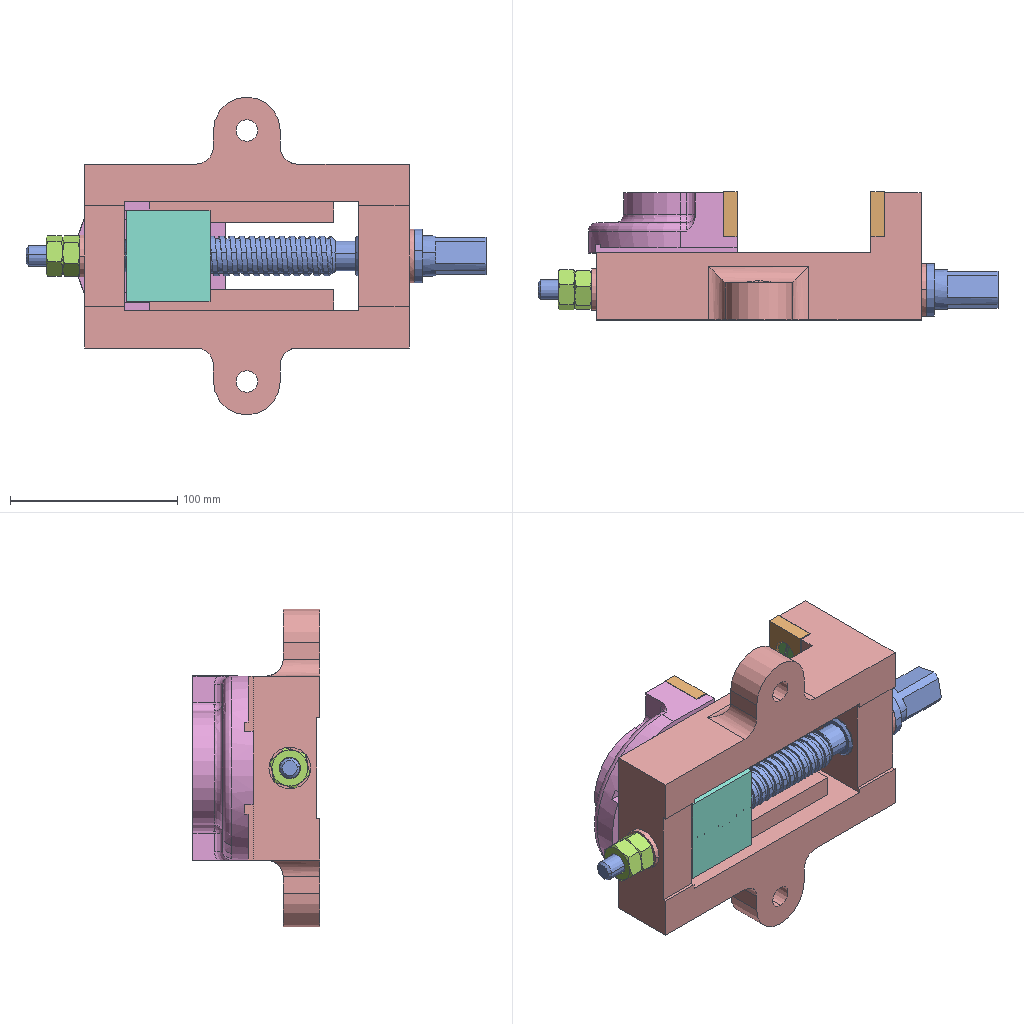Assembly | SolidWorks | 13 different items | 18 placed | box 275 x 76 x 190 mm
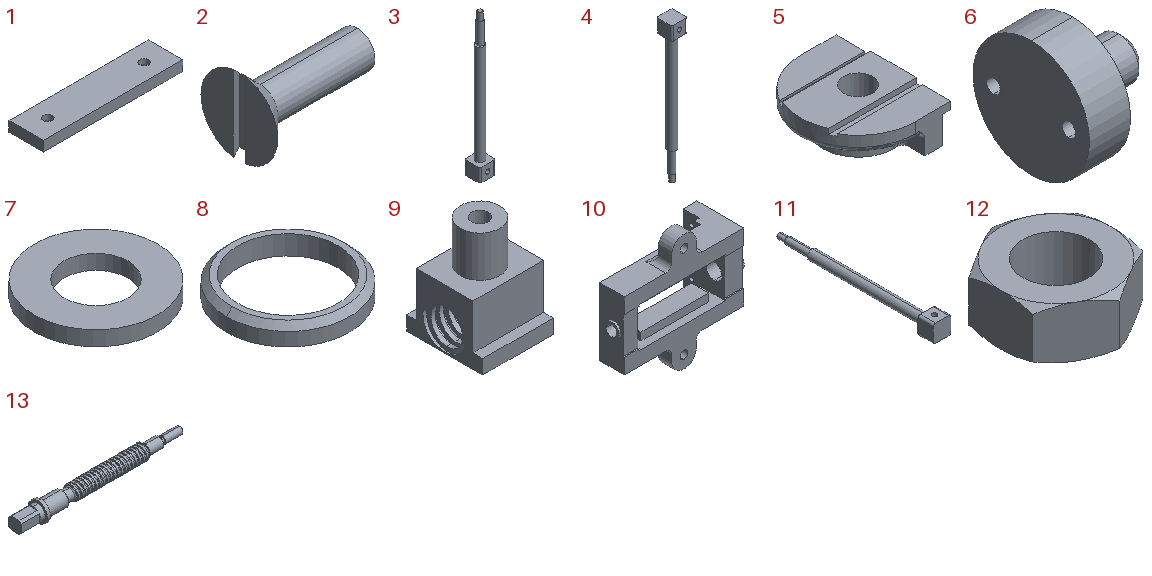Parts list (item | quantity | size | volume | features):
1 | x2 | 110 x 27 x 8 mm | 22658 mm3 | features Extrusion 1, MirrorPattern 1, RevCut 1
2 | x4 | 21.732 x 13 x 12.845 mm | 718.275 mm3 | features ICE 1, Revolution 1
3 | x1 | 40 x 40 x 370 mm | 162246 mm3 | features ICE 4, Chamfer 1, Extrusion 1
4 | x1 | 40 x 40 x 370 mm | 162450 mm3 | features ICE 4, Chamfer 1, Extrusion 1
5 | x1 | 89 x 110 x 36 mm | 178955 mm3 | features ICE 6, Fillet 3, Extrusion 1, MirrorPattern 1, RevCut 1
6 | x1 | 27 x 34 x 34 mm | 12223 mm3 | features Chamfer 1, MirrorPattern 1, RevCut 1, Revolution 1
7 | x1 | 25 x 25 x 3 mm | 1074 mm3 | features Extrusion 1
8 | x1 | 32 x 32 x 5 mm | 1257 mm3 | features Chamfer 1, Extrusion 1
9 | x1 | 50 x 54 x 71 mm | 75271 mm3 | features ICE 3, Extrusion 1, Helix 1, RevCut 1, SweepCut 1
10 | x1 | 200 x 76 x 190 mm | 696258 mm3 | features ICE 10, Extrusion 1, Fillet 1, MirrorSolid 1
11 | x1 | 40 x 370 x 40 mm | 162246 mm3 | features ICE 4, Chamfer 1, Extrusion 1
12 | x2 | 21.651 x 25 x 10 mm | 2710 mm3 | features ICE 2, Extrusion 1, MirrorPattern 1
13 | x1 | 275 x 32 x 32 mm | 98035 mm3 | features Chamfer 2, ICE 2, Helix 1, Revolution 1, SweepCut 1
Mates (type | each side: item.copy, entity, surface, feature):
Concentric | 10.1 face cylinder Cut-Extrude2 | 13.1 face cylinder Revolve1
Coincident | 10.1 face plane Boss-Extrude2 | 13.1 face plane Revolve1
Concentric | 13.1 face cylinder Revolve1 | 12.1 face cylinder Cut-Extrude2
Coincident | 10.1 face plane Boss-Extrude3 | 12.1 face plane Boss-Extrude1
Concentric | 13.1 face cylinder Revolve1 | 12.2 face cylinder Cut-Extrude2
Coincident | 12.1 face plane Boss-Extrude1 | 12.2 face plane Boss-Extrude1
Coincident | 10.1 face plane Cut-Extrude7 | 9.1 face plane Boss-Extrude1
Coincident | 10.1 face plane Cut-Extrude4 | 9.1 face plane Boss-Extrude2
Coincident | 10.1 face plane Boss-Extrude1 | 1.1 face plane Boss-Extrude1
Concentric | 10.1 face cylinder Cut-Extrude8 | 1.1 face cylinder Cut-Revolve2
Concentric | 10.1 face cylinder Cut-Extrude8 | 1.1 edge
Concentric | 5.1 face cylinder Cut-Extrude1 | 9.1 face cylinder Boss-Extrude3
Coincident | 10.1 face plane Boss-Extrude1 | 5.1 face plane Boss-Extrude1 | 2 times
Concentric | 5.1 face cylinder Mirror1 | 1.2 face cylinder Cut-Revolve2
Concentric | 5.1 face cylinder Cut-Revolve2 | 1.2 face cylinder Mirror1
Coincident | 5.1 face plane Boss-Extrude3 | 1.2 face plane Boss-Extrude1
Concentric | 9.1 face cylinder Cut-Revolve1 | 6.1 face cylinder Revolve1
Coincident | 5.1 face plane Cut-Extrude2 | 6.1 face plane Revolve1
Concentric | 5.1 face cylinder Mirror1 | 2.1 face cylinder Revolve1
Coincident | 1.2 face cone Cut-Revolve2 | 2.1 face cone Revolve1
Concentric | 1.2 face cylinder Mirror1 | 2.2 face cylinder Revolve1
Coincident | 1.2 face cone Mirror1 | 2.2 face cone Revolve1
Concentric | 1.1 face cylinder Mirror1 | 2.3 face cylinder Revolve1
Concentric | 1.1 face cylinder Cut-Revolve2 | 2.4 face cylinder Revolve1
Coincident | 1.1 face cone Mirror1 | 2.3 face cone Revolve1
Coincident | 1.1 face cone Cut-Revolve2 | 2.4 face cone Revolve1
LimitDistanceDim | 1.2 face plane Boss-Extrude1 | 1.1 face plane Boss-Extrude1
Screw | 10.1 face cylinder Cut-Extrude2 | 13.1 face cylinder Revolve1